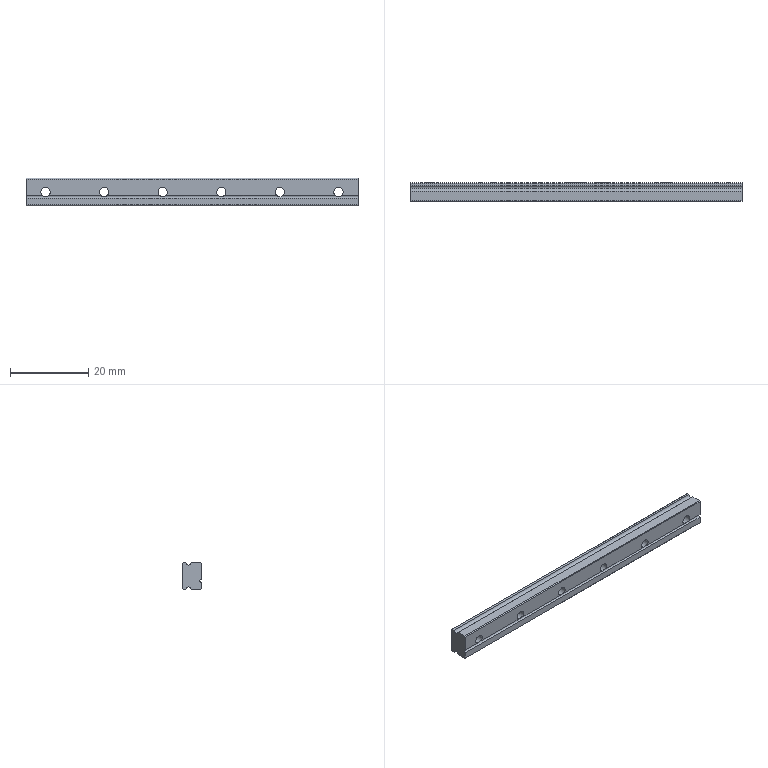Part | SolidWorks | features BaseBody 1, LPattern 1, MoveFace 1 | 1 solid | 170 faces | box 85 x 4.8 x 7 mm | volume 2439 mm3 | plane 85 | spline 57 | cylinder 28 | commonest cylinder face diameters 2.4 x12 4.2 x12 1.4 x3 0.8 x1